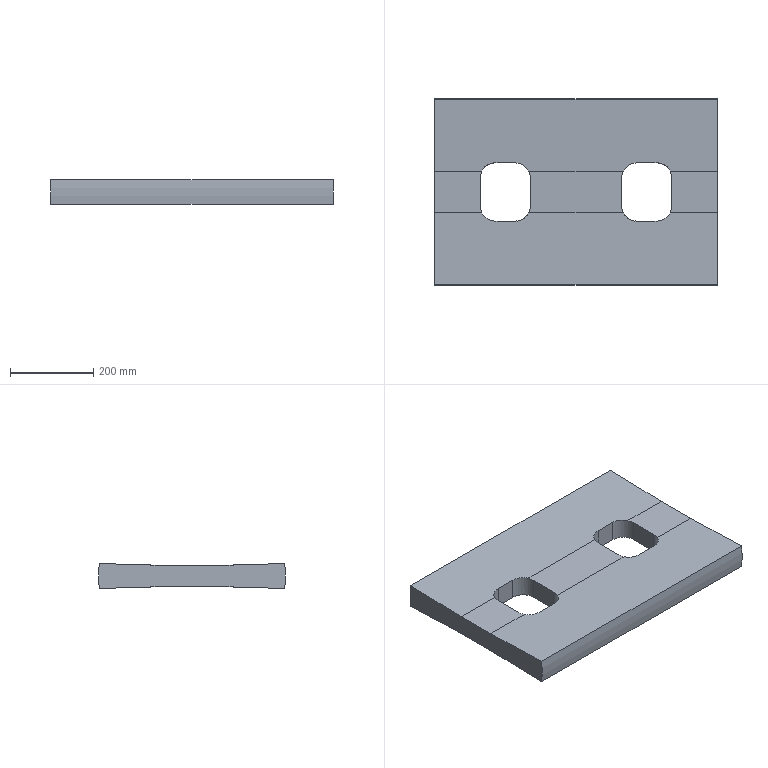Part | SolidWorks | features Extrusion 1, ICE 1, MirrorPattern 1 | 1 solid | 30 faces | box 680 x 450 x 60 mm | volume 14870230 mm3 | plane 20 | cylinder 10 | commonest cylinder face diameters 70 x8 450 x2
STEP:
#1=CARTESIAN_POINT('',(110.,-35.,25.));
#2=VERTEX_POINT('',#1);
#3=CARTESIAN_POINT('',(113.377,-50.,25.));
#4=VERTEX_POINT('',#3);
#5=CARTESIAN_POINT('',(145.,-35.,25.));
#6=DIRECTION('',(0.,0.,1.));
#7=DIRECTION('',(0.,1.,0.));
#8=AXIS2_PLACEMENT_3D('',#5,#6,#7);
#9=CIRCLE('',#8,35.);
#10=EDGE_CURVE('',#2,#4,#9,.T.);
#11=ORIENTED_EDGE('',*,*,#10,.F.);
#12=CARTESIAN_POINT('',(110.,35.,25.));
#13=VERTEX_POINT('',#12);
#14=CARTESIAN_POINT('',(110.,-50.,25.));
#15=DIRECTION('',(0.,-1.,0.));
#16=VECTOR('',#15,1000.);
#17=LINE('',#14,#16);
#18=EDGE_CURVE('',#13,#2,#17,.T.);
#19=ORIENTED_EDGE('',*,*,#18,.F.);
#20=CARTESIAN_POINT('',(113.377,50.,25.));
#21=VERTEX_POINT('',#20);
#22=CARTESIAN_POINT('',(145.,35.,25.));
#23=DIRECTION('',(0.,0.,1.));
#24=DIRECTION('',(0.,1.,0.));
#25=AXIS2_PLACEMENT_3D('',#22,#23,#24);
#26=CIRCLE('',#25,35.);
#27=EDGE_CURVE('',#21,#13,#26,.T.);
#28=ORIENTED_EDGE('',*,*,#27,.F.);
#29=CARTESIAN_POINT('',(-113.377,50.,25.));
#30=VERTEX_POINT('',#29);
#31=CARTESIAN_POINT('',(340.,50.,25.));
#32=DIRECTION('',(-1.,0.,0.));
#33=VECTOR('',#32,1000.);
#34=LINE('',#31,#33);
#35=EDGE_CURVE('',#21,#30,#34,.T.);
#36=ORIENTED_EDGE('',*,*,#35,.T.);
#37=CARTESIAN_POINT('',(-110.,35.,25.));
#38=VERTEX_POINT('',#37);
#39=CARTESIAN_POINT('',(-145.,35.,25.));
#40=DIRECTION('',(0.,0.,-1.));
#41=DIRECTION('',(0.,1.,0.));
#42=AXIS2_PLACEMENT_3D('',#39,#40,#41);
#43=CIRCLE('',#42,35.);
#44=EDGE_CURVE('',#30,#38,#43,.T.);
#45=ORIENTED_EDGE('',*,*,#44,.T.);
#46=CARTESIAN_POINT('',(-110.,-35.,25.));
#47=VERTEX_POINT('',#46);
#48=CARTESIAN_POINT('',(-110.,-50.,25.));
#49=DIRECTION('',(0.,-1.,0.));
#50=VECTOR('',#49,1000.);
#51=LINE('',#48,#50);
#52=EDGE_CURVE('',#38,#47,#51,.T.);
#53=ORIENTED_EDGE('',*,*,#52,.T.);
#54=CARTESIAN_POINT('',(-113.377,-50.,25.));
#55=VERTEX_POINT('',#54);
#56=CARTESIAN_POINT('',(-145.,-35.,25.));
#57=DIRECTION('',(0.,0.,-1.));
#58=DIRECTION('',(0.,1.,0.));
#59=AXIS2_PLACEMENT_3D('',#56,#57,#58);
#60=CIRCLE('',#59,35.);
#61=EDGE_CURVE('',#47,#55,#60,.T.);
#62=ORIENTED_EDGE('',*,*,#61,.T.);
#63=CARTESIAN_POINT('',(340.,-50.,25.));
#64=DIRECTION('',(-1.,0.,0.));
#65=VECTOR('',#64,1000.);
#66=LINE('',#63,#65);
#67=EDGE_CURVE('',#4,#55,#66,.T.);
#68=ORIENTED_EDGE('',*,*,#67,.F.);
#69=EDGE_LOOP('',(#11,#19,#28,#36,#45,#53,#62,#68));
#70=FACE_OUTER_BOUND('',#69,.T.);
#71=CARTESIAN_POINT('',(340.,-50.,25.));
#72=DIRECTION('',(0.,0.,-1.));
#73=DIRECTION('',(0.,1.,0.));
#74=AXIS2_PLACEMENT_3D('',#71,#72,#73);
#75=PLANE('',#74);
#76=ADVANCED_FACE('',(#70),#75,.F.);
#77=CARTESIAN_POINT('',(145.,-70.,25.578));
#78=VERTEX_POINT('',#77);
#79=CARTESIAN_POINT('',(113.377,-50.,25.));
#80=CARTESIAN_POINT('',(119.338,-62.566,25.363));
#81=CARTESIAN_POINT('',(131.092,-70.,25.578));
#82=CARTESIAN_POINT('',(145.,-70.,25.578));
#83=(BOUNDED_CURVE()B_SPLINE_CURVE(3,(#79,#80,#81,#82),.UNSPECIFIED.,.F.,.F.)B_SPLINE_CURVE_WITH_KNOTS((4,4),(5.155,6.283),.UNSPECIFIED.)CURVE()GEOMETRIC_REPRESENTATION_ITEM()RATIONAL_B_SPLINE_CURVE((1.,0.8968,0.8968,1.))REPRESENTATION_ITEM(''));
#84=EDGE_CURVE('',#4,#78,#83,.T.);
#85=ORIENTED_EDGE('',*,*,#84,.F.);
#86=ORIENTED_EDGE('',*,*,#67,.T.);
#87=CARTESIAN_POINT('',(-145.,-70.,25.578));
#88=VERTEX_POINT('',#87);
#89=CARTESIAN_POINT('',(-113.377,-50.,25.));
#90=CARTESIAN_POINT('',(-119.338,-62.566,25.363));
#91=CARTESIAN_POINT('',(-131.092,-70.,25.578));
#92=CARTESIAN_POINT('',(-145.,-70.,25.578));
#93=(BOUNDED_CURVE()B_SPLINE_CURVE(3,(#89,#90,#91,#92),.UNSPECIFIED.,.F.,.F.)B_SPLINE_CURVE_WITH_KNOTS((4,4),(5.155,6.283),.UNSPECIFIED.)CURVE()GEOMETRIC_REPRESENTATION_ITEM()RATIONAL_B_SPLINE_CURVE((1.,0.8968,0.8968,1.))REPRESENTATION_ITEM(''));
#94=EDGE_CURVE('',#55,#88,#93,.T.);
#95=ORIENTED_EDGE('',*,*,#94,.T.);
#96=CARTESIAN_POINT('',(-195.,-70.,25.578));
#97=VERTEX_POINT('',#96);
#98=CARTESIAN_POINT('',(340.,-70.,25.578));
#99=DIRECTION('',(-1.,0.,0.));
#100=VECTOR('',#99,1000.);
#101=LINE('',#98,#100);
#102=EDGE_CURVE('',#88,#97,#101,.T.);
#103=ORIENTED_EDGE('',*,*,#102,.T.);
#104=CARTESIAN_POINT('',(-226.623,-50.,25.));
#105=VERTEX_POINT('',#104);
#106=CARTESIAN_POINT('',(-195.,-70.,25.578));
#107=CARTESIAN_POINT('',(-208.908,-70.,25.578));
#108=CARTESIAN_POINT('',(-220.662,-62.566,25.363));
#109=CARTESIAN_POINT('',(-226.623,-50.,25.));
#110=(BOUNDED_CURVE()B_SPLINE_CURVE(3,(#106,#107,#108,#109),.UNSPECIFIED.,.F.,.F.)B_SPLINE_CURVE_WITH_KNOTS((4,4),(0.,1.128),.UNSPECIFIED.)CURVE()GEOMETRIC_REPRESENTATION_ITEM()RATIONAL_B_SPLINE_CURVE((1.,0.8968,0.8968,1.))REPRESENTATION_ITEM(''));
#111=EDGE_CURVE('',#97,#105,#110,.T.);
#112=ORIENTED_EDGE('',*,*,#111,.T.);
#113=CARTESIAN_POINT('',(-340.,-50.,25.));
#114=VERTEX_POINT('',#113);
#115=CARTESIAN_POINT('',(340.,-50.,25.));
#116=DIRECTION('',(-1.,0.,0.));
#117=VECTOR('',#116,1000.);
#118=LINE('',#115,#117);
#119=EDGE_CURVE('',#105,#114,#118,.T.);
#120=ORIENTED_EDGE('',*,*,#119,.T.);
#121=CARTESIAN_POINT('',(-340.,-222.991,30.));
#122=VERTEX_POINT('',#121);
#123=CARTESIAN_POINT('',(-340.,-50.,25.));
#124=DIRECTION('',(0.,-0.9996,0.02889));
#125=VECTOR('',#124,1000.);
#126=LINE('',#123,#125);
#127=EDGE_CURVE('',#114,#122,#126,.T.);
#128=ORIENTED_EDGE('',*,*,#127,.T.);
#129=CARTESIAN_POINT('',(340.,-222.991,30.));
#130=VERTEX_POINT('',#129);
#131=CARTESIAN_POINT('',(340.,-222.991,30.));
#132=DIRECTION('',(-1.,0.,0.));
#133=VECTOR('',#132,1000.);
#134=LINE('',#131,#133);
#135=EDGE_CURVE('',#130,#122,#134,.T.);
#136=ORIENTED_EDGE('',*,*,#135,.F.);
#137=CARTESIAN_POINT('',(340.,-50.,25.));
#138=VERTEX_POINT('',#137);
#139=CARTESIAN_POINT('',(340.,-50.,25.));
#140=DIRECTION('',(0.,-0.9996,0.02889));
#141=VECTOR('',#140,1000.);
#142=LINE('',#139,#141);
#143=EDGE_CURVE('',#138,#130,#142,.T.);
#144=ORIENTED_EDGE('',*,*,#143,.F.);
#145=CARTESIAN_POINT('',(226.623,-50.,25.));
#146=VERTEX_POINT('',#145);
#147=CARTESIAN_POINT('',(340.,-50.,25.));
#148=DIRECTION('',(-1.,0.,0.));
#149=VECTOR('',#148,1000.);
#150=LINE('',#147,#149);
#151=EDGE_CURVE('',#138,#146,#150,.T.);
#152=ORIENTED_EDGE('',*,*,#151,.T.);
#153=CARTESIAN_POINT('',(195.,-70.,25.578));
#154=VERTEX_POINT('',#153);
#155=CARTESIAN_POINT('',(195.,-70.,25.578));
#156=CARTESIAN_POINT('',(208.908,-70.,25.578));
#157=CARTESIAN_POINT('',(220.662,-62.566,25.363));
#158=CARTESIAN_POINT('',(226.623,-50.,25.));
#159=(BOUNDED_CURVE()B_SPLINE_CURVE(3,(#155,#156,#157,#158),.UNSPECIFIED.,.F.,.F.)B_SPLINE_CURVE_WITH_KNOTS((4,4),(0.,1.128),.UNSPECIFIED.)CURVE()GEOMETRIC_REPRESENTATION_ITEM()RATIONAL_B_SPLINE_CURVE((1.,0.8968,0.8968,1.))REPRESENTATION_ITEM(''));
#160=EDGE_CURVE('',#154,#146,#159,.T.);
#161=ORIENTED_EDGE('',*,*,#160,.F.);
#162=CARTESIAN_POINT('',(340.,-70.,25.578));
#163=DIRECTION('',(1.,0.,0.));
#164=VECTOR('',#163,1000.);
#165=LINE('',#162,#164);
#166=EDGE_CURVE('',#78,#154,#165,.T.);
#167=ORIENTED_EDGE('',*,*,#166,.F.);
#168=EDGE_LOOP('',(#85,#86,#95,#103,#112,#120,#128,#136,#144,#152,#161,#167));
#169=FACE_OUTER_BOUND('',#168,.T.);
#170=CARTESIAN_POINT('',(340.,-50.,25.));
#171=DIRECTION('',(0.,-0.02889,-0.9996));
#172=DIRECTION('',(0.,0.9996,-0.02889));
#173=AXIS2_PLACEMENT_3D('',#170,#171,#172);
#174=PLANE('',#173);
#175=ADVANCED_FACE('',(#169),#174,.F.);
#176=CARTESIAN_POINT('',(145.,-70.,-25.578));
#177=VERTEX_POINT('',#176);
#178=CARTESIAN_POINT('',(113.377,-50.,-25.));
#179=VERTEX_POINT('',#178);
#180=CARTESIAN_POINT('',(145.,-70.,-25.578));
#181=CARTESIAN_POINT('',(131.092,-70.,-25.578));
#182=CARTESIAN_POINT('',(119.338,-62.566,-25.363));
#183=CARTESIAN_POINT('',(113.377,-50.,-25.));
#184=(BOUNDED_CURVE()B_SPLINE_CURVE(3,(#180,#181,#182,#183),.UNSPECIFIED.,.F.,.T.)B_SPLINE_CURVE_WITH_KNOTS((4,4),(3.142,4.269),.UNSPECIFIED.)CURVE()GEOMETRIC_REPRESENTATION_ITEM()RATIONAL_B_SPLINE_CURVE((1.,0.8968,0.8968,1.))REPRESENTATION_ITEM(''));
#185=EDGE_CURVE('',#177,#179,#184,.T.);
#186=ORIENTED_EDGE('',*,*,#185,.F.);
#187=CARTESIAN_POINT('',(195.,-70.,-25.578));
#188=VERTEX_POINT('',#187);
#189=CARTESIAN_POINT('',(340.,-70.,-25.578));
#190=DIRECTION('',(-1.,0.,0.));
#191=VECTOR('',#190,1000.);
#192=LINE('',#189,#191);
#193=EDGE_CURVE('',#188,#177,#192,.T.);
#194=ORIENTED_EDGE('',*,*,#193,.F.);
#195=CARTESIAN_POINT('',(226.623,-50.,-25.));
#196=VERTEX_POINT('',#195);
#197=CARTESIAN_POINT('',(226.623,-50.,-25.));
#198=CARTESIAN_POINT('',(220.662,-62.566,-25.363));
#199=CARTESIAN_POINT('',(208.908,-70.,-25.578));
#200=CARTESIAN_POINT('',(195.,-70.,-25.578));
#201=(BOUNDED_CURVE()B_SPLINE_CURVE(3,(#197,#198,#199,#200),.UNSPECIFIED.,.F.,.F.)B_SPLINE_CURVE_WITH_KNOTS((4,4),(2.014,3.142),.UNSPECIFIED.)CURVE()GEOMETRIC_REPRESENTATION_ITEM()RATIONAL_B_SPLINE_CURVE((1.,0.8968,0.8968,1.))REPRESENTATION_ITEM(''));
#202=EDGE_CURVE('',#196,#188,#201,.T.);
#203=ORIENTED_EDGE('',*,*,#202,.F.);
#204=CARTESIAN_POINT('',(340.,-50.,-25.));
#205=VERTEX_POINT('',#204);
#206=CARTESIAN_POINT('',(340.,-50.,-25.));
#207=DIRECTION('',(-1.,0.,0.));
#208=VECTOR('',#207,1000.);
#209=LINE('',#206,#208);
#210=EDGE_CURVE('',#205,#196,#209,.T.);
#211=ORIENTED_EDGE('',*,*,#210,.F.);
#212=CARTESIAN_POINT('',(340.,-222.991,-30.));
#213=VERTEX_POINT('',#212);
#214=CARTESIAN_POINT('',(340.,-50.,-25.));
#215=DIRECTION('',(0.,0.9996,0.02889));
#216=VECTOR('',#215,1000.);
#217=LINE('',#214,#216);
#218=EDGE_CURVE('',#213,#205,#217,.T.);
#219=ORIENTED_EDGE('',*,*,#218,.F.);
#220=CARTESIAN_POINT('',(-340.,-222.991,-30.));
#221=VERTEX_POINT('',#220);
#222=CARTESIAN_POINT('',(340.,-222.991,-30.));
#223=DIRECTION('',(-1.,0.,0.));
#224=VECTOR('',#223,1000.);
#225=LINE('',#222,#224);
#226=EDGE_CURVE('',#213,#221,#225,.T.);
#227=ORIENTED_EDGE('',*,*,#226,.T.);
#228=CARTESIAN_POINT('',(-340.,-50.,-25.));
#229=VERTEX_POINT('',#228);
#230=CARTESIAN_POINT('',(-340.,-50.,-25.));
#231=DIRECTION('',(0.,0.9996,0.02889));
#232=VECTOR('',#231,1000.);
#233=LINE('',#230,#232);
#234=EDGE_CURVE('',#221,#229,#233,.T.);
#235=ORIENTED_EDGE('',*,*,#234,.T.);
#236=CARTESIAN_POINT('',(-226.623,-50.,-25.));
#237=VERTEX_POINT('',#236);
#238=CARTESIAN_POINT('',(340.,-50.,-25.));
#239=DIRECTION('',(-1.,0.,0.));
#240=VECTOR('',#239,1000.);
#241=LINE('',#238,#240);
#242=EDGE_CURVE('',#237,#229,#241,.T.);
#243=ORIENTED_EDGE('',*,*,#242,.F.);
#244=CARTESIAN_POINT('',(-195.,-70.,-25.578));
#245=VERTEX_POINT('',#244);
#246=CARTESIAN_POINT('',(-226.623,-50.,-25.));
#247=CARTESIAN_POINT('',(-220.662,-62.566,-25.363));
#248=CARTESIAN_POINT('',(-208.908,-70.,-25.578));
#249=CARTESIAN_POINT('',(-195.,-70.,-25.578));
#250=(BOUNDED_CURVE()B_SPLINE_CURVE(3,(#246,#247,#248,#249),.UNSPECIFIED.,.F.,.F.)B_SPLINE_CURVE_WITH_KNOTS((4,4),(2.014,3.142),.UNSPECIFIED.)CURVE()GEOMETRIC_REPRESENTATION_ITEM()RATIONAL_B_SPLINE_CURVE((1.,0.8968,0.8968,1.))REPRESENTATION_ITEM(''));
#251=EDGE_CURVE('',#237,#245,#250,.T.);
#252=ORIENTED_EDGE('',*,*,#251,.T.);
#253=CARTESIAN_POINT('',(-145.,-70.,-25.578));
#254=VERTEX_POINT('',#253);
#255=CARTESIAN_POINT('',(340.,-70.,-25.578));
#256=DIRECTION('',(1.,0.,0.));
#257=VECTOR('',#256,1000.);
#258=LINE('',#255,#257);
#259=EDGE_CURVE('',#245,#254,#258,.T.);
#260=ORIENTED_EDGE('',*,*,#259,.T.);
#261=CARTESIAN_POINT('',(-113.377,-50.,-25.));
#262=VERTEX_POINT('',#261);
#263=CARTESIAN_POINT('',(-145.,-70.,-25.578));
#264=CARTESIAN_POINT('',(-131.092,-70.,-25.578));
#265=CARTESIAN_POINT('',(-119.338,-62.566,-25.363));
#266=CARTESIAN_POINT('',(-113.377,-50.,-25.));
#267=(BOUNDED_CURVE()B_SPLINE_CURVE(3,(#263,#264,#265,#266),.UNSPECIFIED.,.F.,.T.)B_SPLINE_CURVE_WITH_KNOTS((4,4),(3.142,4.269),.UNSPECIFIED.)CURVE()GEOMETRIC_REPRESENTATION_ITEM()RATIONAL_B_SPLINE_CURVE((1.,0.8968,0.8968,1.))REPRESENTATION_ITEM(''));
#268=EDGE_CURVE('',#254,#262,#267,.T.);
#269=ORIENTED_EDGE('',*,*,#268,.T.);
#270=CARTESIAN_POINT('',(340.,-50.,-25.));
#271=DIRECTION('',(-1.,0.,0.));
#272=VECTOR('',#271,1000.);
#273=LINE('',#270,#272);
#274=EDGE_CURVE('',#179,#262,#273,.T.);
#275=ORIENTED_EDGE('',*,*,#274,.F.);
#276=EDGE_LOOP('',(#186,#194,#203,#211,#219,#227,#235,#243,#252,#260,#269,#275));
#277=FACE_OUTER_BOUND('',#276,.T.);
#278=CARTESIAN_POINT('',(340.,-50.,-25.));
#279=DIRECTION('',(0.,-0.02889,0.9996));
#280=DIRECTION('',(0.,-0.9996,-0.02889));
#281=AXIS2_PLACEMENT_3D('',#278,#279,#280);
#282=PLANE('',#281);
#283=ADVANCED_FACE('',(#277),#282,.F.);
#284=CARTESIAN_POINT('',(110.,-35.,-25.));
#285=VERTEX_POINT('',#284);
#286=CARTESIAN_POINT('',(145.,-35.,-25.));
#287=DIRECTION('',(0.,0.,-1.));
#288=DIRECTION('',(0.,-1.,0.));
#289=AXIS2_PLACEMENT_3D('',#286,#287,#288);
#290=CIRCLE('',#289,35.);
#291=EDGE_CURVE('',#179,#285,#290,.T.);
#292=ORIENTED_EDGE('',*,*,#291,.F.);
#293=ORIENTED_EDGE('',*,*,#274,.T.);
#294=CARTESIAN_POINT('',(-110.,-35.,-25.));
#295=VERTEX_POINT('',#294);
#296=CARTESIAN_POINT('',(-145.,-35.,-25.));
#297=DIRECTION('',(0.,0.,1.));
#298=DIRECTION('',(0.,-1.,0.));
#299=AXIS2_PLACEMENT_3D('',#296,#297,#298);
#300=CIRCLE('',#299,35.);
#301=EDGE_CURVE('',#262,#295,#300,.T.);
#302=ORIENTED_EDGE('',*,*,#301,.T.);
#303=CARTESIAN_POINT('',(-110.,35.,-25.));
#304=VERTEX_POINT('',#303);
#305=CARTESIAN_POINT('',(-110.,-50.,-25.));
#306=DIRECTION('',(0.,1.,0.));
#307=VECTOR('',#306,1000.);
#308=LINE('',#305,#307);
#309=EDGE_CURVE('',#295,#304,#308,.T.);
#310=ORIENTED_EDGE('',*,*,#309,.T.);
#311=CARTESIAN_POINT('',(-113.377,50.,-25.));
#312=VERTEX_POINT('',#311);
#313=CARTESIAN_POINT('',(-145.,35.,-25.));
#314=DIRECTION('',(0.,0.,1.));
#315=DIRECTION('',(0.,-1.,0.));
#316=AXIS2_PLACEMENT_3D('',#313,#314,#315);
#317=CIRCLE('',#316,35.);
#318=EDGE_CURVE('',#304,#312,#317,.T.);
#319=ORIENTED_EDGE('',*,*,#318,.T.);
#320=CARTESIAN_POINT('',(113.377,50.,-25.));
#321=VERTEX_POINT('',#320);
#322=CARTESIAN_POINT('',(340.,50.,-25.));
#323=DIRECTION('',(-1.,0.,0.));
#324=VECTOR('',#323,1000.);
#325=LINE('',#322,#324);
#326=EDGE_CURVE('',#321,#312,#325,.T.);
#327=ORIENTED_EDGE('',*,*,#326,.F.);
#328=CARTESIAN_POINT('',(110.,35.,-25.));
#329=VERTEX_POINT('',#328);
#330=CARTESIAN_POINT('',(145.,35.,-25.));
#331=DIRECTION('',(0.,0.,-1.));
#332=DIRECTION('',(0.,-1.,0.));
#333=AXIS2_PLACEMENT_3D('',#330,#331,#332);
#334=CIRCLE('',#333,35.);
#335=EDGE_CURVE('',#329,#321,#334,.T.);
#336=ORIENTED_EDGE('',*,*,#335,.F.);
#337=CARTESIAN_POINT('',(110.,-50.,-25.));
#338=DIRECTION('',(0.,1.,0.));
#339=VECTOR('',#338,1000.);
#340=LINE('',#337,#339);
#341=EDGE_CURVE('',#285,#329,#340,.T.);
#342=ORIENTED_EDGE('',*,*,#341,.F.);
#343=EDGE_LOOP('',(#292,#293,#302,#310,#319,#327,#336,#342));
#344=FACE_OUTER_BOUND('',#343,.T.);
#345=CARTESIAN_POINT('',(340.,-50.,-25.));
#346=DIRECTION('',(0.,0.,1.));
#347=DIRECTION('',(0.,-1.,0.));
#348=AXIS2_PLACEMENT_3D('',#345,#346,#347);
#349=PLANE('',#348);
#350=ADVANCED_FACE('',(#344),#349,.F.);
#351=ORIENTED_EDGE('',*,*,#119,.F.);
#352=CARTESIAN_POINT('',(-230.,-35.,25.));
#353=VERTEX_POINT('',#352);
#354=CARTESIAN_POINT('',(-195.,-35.,25.));
#355=DIRECTION('',(0.,0.,-1.));
#356=DIRECTION('',(0.,1.,0.));
#357=AXIS2_PLACEMENT_3D('',#354,#355,#356);
#358=CIRCLE('',#357,35.);
#359=EDGE_CURVE('',#105,#353,#358,.T.);
#360=ORIENTED_EDGE('',*,*,#359,.T.);
#361=CARTESIAN_POINT('',(-230.,35.,25.));
#362=VERTEX_POINT('',#361);
#363=CARTESIAN_POINT('',(-230.,-50.,25.));
#364=DIRECTION('',(0.,1.,0.));
#365=VECTOR('',#364,1000.);
#366=LINE('',#363,#365);
#367=EDGE_CURVE('',#353,#362,#366,.T.);
#368=ORIENTED_EDGE('',*,*,#367,.T.);
#369=CARTESIAN_POINT('',(-226.623,50.,25.));
#370=VERTEX_POINT('',#369);
#371=CARTESIAN_POINT('',(-195.,35.,25.));
#372=DIRECTION('',(0.,0.,-1.));
#373=DIRECTION('',(0.,1.,0.));
#374=AXIS2_PLACEMENT_3D('',#371,#372,#373);
#375=CIRCLE('',#374,35.);
#376=EDGE_CURVE('',#362,#370,#375,.T.);
#377=ORIENTED_EDGE('',*,*,#376,.T.);
#378=CARTESIAN_POINT('',(-340.,50.,25.));
#379=VERTEX_POINT('',#378);
#380=CARTESIAN_POINT('',(340.,50.,25.));
#381=DIRECTION('',(-1.,0.,0.));
#382=VECTOR('',#381,1000.);
#383=LINE('',#380,#382);
#384=EDGE_CURVE('',#370,#379,#383,.T.);
#385=ORIENTED_EDGE('',*,*,#384,.T.);
#386=CARTESIAN_POINT('',(-340.,-50.,25.));
#387=DIRECTION('',(0.,-1.,0.));
#388=VECTOR('',#387,1000.);
#389=LINE('',#386,#388);
#390=EDGE_CURVE('',#379,#114,#389,.T.);
#391=ORIENTED_EDGE('',*,*,#390,.T.);
#392=EDGE_LOOP('',(#351,#360,#368,#377,#385,#391));
#393=FACE_OUTER_BOUND('',#392,.T.);
#394=CARTESIAN_POINT('',(340.,-50.,25.));
#395=DIRECTION('',(0.,0.,-1.));
#396=DIRECTION('',(0.,1.,0.));
#397=AXIS2_PLACEMENT_3D('',#394,#395,#396);
#398=PLANE('',#397);
#399=ADVANCED_FACE('',(#393),#398,.F.);
#400=CARTESIAN_POINT('',(-230.,35.,-25.));
#401=VERTEX_POINT('',#400);
#402=CARTESIAN_POINT('',(-230.,-35.,-25.));
#403=VERTEX_POINT('',#402);
#404=CARTESIAN_POINT('',(-230.,-50.,-25.));
#405=DIRECTION('',(0.,-1.,0.));
#406=VECTOR('',#405,1000.);
#407=LINE('',#404,#406);
#408=EDGE_CURVE('',#401,#403,#407,.T.);
#409=ORIENTED_EDGE('',*,*,#408,.T.);
#410=CARTESIAN_POINT('',(-195.,-35.,-25.));
#411=DIRECTION('',(0.,0.,1.));
#412=DIRECTION('',(0.,-1.,0.));
#413=AXIS2_PLACEMENT_3D('',#410,#411,#412);
#414=CIRCLE('',#413,35.);
#415=EDGE_CURVE('',#403,#237,#414,.T.);
#416=ORIENTED_EDGE('',*,*,#415,.T.);
#417=ORIENTED_EDGE('',*,*,#242,.T.);
#418=CARTESIAN_POINT('',(-340.,50.,-25.));
#419=VERTEX_POINT('',#418);
#420=CARTESIAN_POINT('',(-340.,-50.,-25.));
#421=DIRECTION('',(0.,1.,0.));
#422=VECTOR('',#421,1000.);
#423=LINE('',#420,#422);
#424=EDGE_CURVE('',#229,#419,#423,.T.);
#425=ORIENTED_EDGE('',*,*,#424,.T.);
#426=CARTESIAN_POINT('',(-226.623,50.,-25.));
#427=VERTEX_POINT('',#426);
#428=CARTESIAN_POINT('',(340.,50.,-25.));
#429=DIRECTION('',(-1.,0.,0.));
#430=VECTOR('',#429,1000.);
#431=LINE('',#428,#430);
#432=EDGE_CURVE('',#427,#419,#431,.T.);
#433=ORIENTED_EDGE('',*,*,#432,.F.);
#434=CARTESIAN_POINT('',(-195.,35.,-25.));
#435=DIRECTION('',(0.,0.,1.));
#436=DIRECTION('',(0.,-1.,0.));
#437=AXIS2_PLACEMENT_3D('',#434,#435,#436);
#438=CIRCLE('',#437,35.);
#439=EDGE_CURVE('',#427,#401,#438,.T.);
#440=ORIENTED_EDGE('',*,*,#439,.T.);
#441=EDGE_LOOP('',(#409,#416,#417,#425,#433,#440));
#442=FACE_OUTER_BOUND('',#441,.T.);
#443=CARTESIAN_POINT('',(340.,-50.,-25.));
#444=DIRECTION('',(0.,0.,1.));
#445=DIRECTION('',(0.,-1.,0.));
#446=AXIS2_PLACEMENT_3D('',#443,#444,#445);
#447=PLANE('',#446);
#448=ADVANCED_FACE('',(#442),#447,.F.);
#449=CARTESIAN_POINT('',(145.,70.,-25.578));
#450=VERTEX_POINT('',#449);
#451=CARTESIAN_POINT('',(113.377,50.,-25.));
#452=CARTESIAN_POINT('',(119.338,62.566,-25.363));
#453=CARTESIAN_POINT('',(131.092,70.,-25.578));
#454=CARTESIAN_POINT('',(145.,70.,-25.578));
#455=(BOUNDED_CURVE()B_SPLINE_CURVE(3,(#451,#452,#453,#454),.UNSPECIFIED.,.F.,.T.)B_SPLINE_CURVE_WITH_KNOTS((4,4),(2.014,3.142),.UNSPECIFIED.)CURVE()GEOMETRIC_REPRESENTATION_ITEM()RATIONAL_B_SPLINE_CURVE((1.,0.8968,0.8968,1.))REPRESENTATION_ITEM(''));
#456=EDGE_CURVE('',#321,#450,#455,.T.);
#457=ORIENTED_EDGE('',*,*,#456,.F.);
#458=ORIENTED_EDGE('',*,*,#326,.T.);
#459=CARTESIAN_POINT('',(-145.,70.,-25.578));
#460=VERTEX_POINT('',#459);
#461=CARTESIAN_POINT('',(-113.377,50.,-25.));
#462=CARTESIAN_POINT('',(-119.338,62.566,-25.363));
#463=CARTESIAN_POINT('',(-131.092,70.,-25.578));
#464=CARTESIAN_POINT('',(-145.,70.,-25.578));
#465=(BOUNDED_CURVE()B_SPLINE_CURVE(3,(#461,#462,#463,#464),.UNSPECIFIED.,.F.,.F.)B_SPLINE_CURVE_WITH_KNOTS((4,4),(2.014,3.142),.UNSPECIFIED.)CURVE()GEOMETRIC_REPRESENTATION_ITEM()RATIONAL_B_SPLINE_CURVE((1.,0.8968,0.8968,1.))REPRESENTATION_ITEM(''));
#466=EDGE_CURVE('',#312,#460,#465,.T.);
#467=ORIENTED_EDGE('',*,*,#466,.T.);
#468=CARTESIAN_POINT('',(-195.,70.,-25.578));
#469=VERTEX_POINT('',#468);
#470=CARTESIAN_POINT('',(340.,70.,-25.578));
#471=DIRECTION('',(-1.,0.,0.));
#472=VECTOR('',#471,1000.);
#473=LINE('',#470,#472);
#474=EDGE_CURVE('',#460,#469,#473,.T.);
#475=ORIENTED_EDGE('',*,*,#474,.T.);
#476=CARTESIAN_POINT('',(-195.,70.,-25.578));
#477=CARTESIAN_POINT('',(-208.908,70.,-25.578));
#478=CARTESIAN_POINT('',(-220.662,62.566,-25.363));
#479=CARTESIAN_POINT('',(-226.623,50.,-25.));
#480=(BOUNDED_CURVE()B_SPLINE_CURVE(3,(#476,#477,#478,#479),.UNSPECIFIED.,.F.,.F.)B_SPLINE_CURVE_WITH_KNOTS((4,4),(3.142,4.269),.UNSPECIFIED.)CURVE()GEOMETRIC_REPRESENTATION_ITEM()RATIONAL_B_SPLINE_CURVE((1.,0.8968,0.8968,1.))REPRESENTATION_ITEM(''));
#481=EDGE_CURVE('',#469,#427,#480,.T.);
#482=ORIENTED_EDGE('',*,*,#481,.T.);
#483=ORIENTED_EDGE('',*,*,#432,.T.);
#484=CARTESIAN_POINT('',(-340.,222.991,-30.));
#485=VERTEX_POINT('',#484);
#486=CARTESIAN_POINT('',(-340.,50.,-25.));
#487=DIRECTION('',(0.,0.9996,-0.02889));
#488=VECTOR('',#487,1000.);
#489=LINE('',#486,#488);
#490=EDGE_CURVE('',#419,#485,#489,.T.);
#491=ORIENTED_EDGE('',*,*,#490,.T.);
#492=CARTESIAN_POINT('',(340.,222.991,-30.));
#493=VERTEX_POINT('',#492);
#494=CARTESIAN_POINT('',(340.,222.991,-30.));
#495=DIRECTION('',(-1.,0.,0.));
#496=VECTOR('',#495,1000.);
#497=LINE('',#494,#496);
#498=EDGE_CURVE('',#493,#485,#497,.T.);
#499=ORIENTED_EDGE('',*,*,#498,.F.);
#500=CARTESIAN_POINT('',(340.,50.,-25.));
#501=VERTEX_POINT('',#500);
#502=CARTESIAN_POINT('',(340.,50.,-25.));
#503=DIRECTION('',(0.,0.9996,-0.02889));
#504=VECTOR('',#503,1000.);
#505=LINE('',#502,#504);
#506=EDGE_CURVE('',#501,#493,#505,.T.);
#507=ORIENTED_EDGE('',*,*,#506,.F.);
#508=CARTESIAN_POINT('',(226.623,50.,-25.));
#509=VERTEX_POINT('',#508);
#510=CARTESIAN_POINT('',(340.,50.,-25.));
#511=DIRECTION('',(-1.,0.,0.));
#512=VECTOR('',#511,1000.);
#513=LINE('',#510,#512);
#514=EDGE_CURVE('',#501,#509,#513,.T.);
#515=ORIENTED_EDGE('',*,*,#514,.T.);
#516=CARTESIAN_POINT('',(195.,70.,-25.578));
#517=VERTEX_POINT('',#516);
#518=CARTESIAN_POINT('',(195.,70.,-25.578));
#519=CARTESIAN_POINT('',(208.908,70.,-25.578));
#520=CARTESIAN_POINT('',(220.662,62.566,-25.363));
#521=CARTESIAN_POINT('',(226.623,50.,-25.));
#522=(BOUNDED_CURVE()B_SPLINE_CURVE(3,(#518,#519,#520,#521),.UNSPECIFIED.,.F.,.T.)B_SPLINE_CURVE_WITH_KNOTS((4,4),(3.142,4.269),.UNSPECIFIED.)CURVE()GEOMETRIC_REPRESENTATION_ITEM()RATIONAL_B_SPLINE_CURVE((1.,0.8968,0.8968,1.))REPRESENTATION_ITEM(''));
#523=EDGE_CURVE('',#517,#509,#522,.T.);
#524=ORIENTED_EDGE('',*,*,#523,.F.);
#525=CARTESIAN_POINT('',(340.,70.,-25.578));
#526=DIRECTION('',(1.,0.,0.));
#527=VECTOR('',#526,1000.);
#528=LINE('',#525,#527);
#529=EDGE_CURVE('',#450,#517,#528,.T.);
#530=ORIENTED_EDGE('',*,*,#529,.F.);
#531=EDGE_LOOP('',(#457,#458,#467,#475,#482,#483,#491,#499,#507,#515,#524,#530));
#532=FACE_OUTER_BOUND('',#531,.T.);
#533=CARTESIAN_POINT('',(340.,50.,-25.));
#534=DIRECTION('',(0.,0.02889,0.9996));
#535=DIRECTION('',(0.,-0.9996,0.02889));
#536=AXIS2_PLACEMENT_3D('',#533,#534,#535);
#537=PLANE('',#536);
#538=ADVANCED_FACE('',(#532),#537,.F.);
#539=CARTESIAN_POINT('',(-340.,222.991,30.));
#540=VERTEX_POINT('',#539);
#541=CARTESIAN_POINT('',(-340.,0.,0.));
#542=DIRECTION('',(1.,0.,0.));
#543=DIRECTION('',(0.,0.,-1.));
#544=AXIS2_PLACEMENT_3D('',#541,#542,#543);
#545=CIRCLE('',#544,225.);
#546=EDGE_CURVE('',#485,#540,#545,.T.);
#547=ORIENTED_EDGE('',*,*,#546,.T.);
#548=CARTESIAN_POINT('',(340.,222.991,30.));
#549=VERTEX_POINT('',#548);
#550=CARTESIAN_POINT('',(340.,222.991,30.));
#551=DIRECTION('',(-1.,0.,0.));
#552=VECTOR('',#551,1000.);
#553=LINE('',#550,#552);
#554=EDGE_CURVE('',#549,#540,#553,.T.);
#555=ORIENTED_EDGE('',*,*,#554,.F.);
#556=CARTESIAN_POINT('',(340.,0.,0.));
#557=DIRECTION('',(1.,0.,0.));
#558=DIRECTION('',(0.,0.,-1.));
#559=AXIS2_PLACEMENT_3D('',#556,#557,#558);
#560=CIRCLE('',#559,225.);
#561=EDGE_CURVE('',#493,#549,#560,.T.);
#562=ORIENTED_EDGE('',*,*,#561,.F.);
#563=ORIENTED_EDGE('',*,*,#498,.T.);
#564=EDGE_LOOP('',(#547,#555,#562,#563));
#565=FACE_OUTER_BOUND('',#564,.T.);
#566=CARTESIAN_POINT('',(340.,0.,0.));
#567=DIRECTION('',(-1.,0.,0.));
#568=DIRECTION('',(0.,0.,1.));
#569=AXIS2_PLACEMENT_3D('',#566,#567,#568);
#570=CYLINDRICAL_SURFACE('',#569,225.);
#571=ADVANCED_FACE('',(#565),#570,.T.);
#572=CARTESIAN_POINT('',(145.,70.,25.578));
#573=VERTEX_POINT('',#572);
#574=CARTESIAN_POINT('',(145.,70.,25.578));
#575=CARTESIAN_POINT('',(131.092,70.,25.578));
#576=CARTESIAN_POINT('',(119.338,62.566,25.363));
#577=CARTESIAN_POINT('',(113.377,50.,25.));
#578=(BOUNDED_CURVE()B_SPLINE_CURVE(3,(#574,#575,#576,#577),.UNSPECIFIED.,.F.,.F.)B_SPLINE_CURVE_WITH_KNOTS((4,4),(0.,1.128),.UNSPECIFIED.)CURVE()GEOMETRIC_REPRESENTATION_ITEM()RATIONAL_B_SPLINE_CURVE((1.,0.8968,0.8968,1.))REPRESENTATION_ITEM(''));
#579=EDGE_CURVE('',#573,#21,#578,.T.);
#580=ORIENTED_EDGE('',*,*,#579,.F.);
#581=CARTESIAN_POINT('',(195.,70.,25.578));
#582=VERTEX_POINT('',#581);
#583=CARTESIAN_POINT('',(340.,70.,25.578));
#584=DIRECTION('',(-1.,0.,0.));
#585=VECTOR('',#584,1000.);
#586=LINE('',#583,#585);
#587=EDGE_CURVE('',#582,#573,#586,.T.);
#588=ORIENTED_EDGE('',*,*,#587,.F.);
#589=CARTESIAN_POINT('',(226.623,50.,25.));
#590=VERTEX_POINT('',#589);
#591=CARTESIAN_POINT('',(226.623,50.,25.));
#592=CARTESIAN_POINT('',(220.662,62.566,25.363));
#593=CARTESIAN_POINT('',(208.908,70.,25.578));
#594=CARTESIAN_POINT('',(195.,70.,25.578));
#595=(BOUNDED_CURVE()B_SPLINE_CURVE(3,(#591,#592,#593,#594),.UNSPECIFIED.,.F.,.F.)B_SPLINE_CURVE_WITH_KNOTS((4,4),(5.155,6.283),.UNSPECIFIED.)CURVE()GEOMETRIC_REPRESENTATION_ITEM()RATIONAL_B_SPLINE_CURVE((1.,0.8968,0.8968,1.))REPRESENTATION_ITEM(''));
#596=EDGE_CURVE('',#590,#582,#595,.T.);
#597=ORIENTED_EDGE('',*,*,#596,.F.);
#598=CARTESIAN_POINT('',(340.,50.,25.));
#599=VERTEX_POINT('',#598);
#600=CARTESIAN_POINT('',(340.,50.,25.));
#601=DIRECTION('',(-1.,0.,0.));
#602=VECTOR('',#601,1000.);
#603=LINE('',#600,#602);
#604=EDGE_CURVE('',#599,#590,#603,.T.);
#605=ORIENTED_EDGE('',*,*,#604,.F.);
#606=CARTESIAN_POINT('',(340.,50.,25.));
#607=DIRECTION('',(0.,-0.9996,-0.02889));
#608=VECTOR('',#607,1000.);
#609=LINE('',#606,#608);
#610=EDGE_CURVE('',#549,#599,#609,.T.);
#611=ORIENTED_EDGE('',*,*,#610,.F.);
#612=ORIENTED_EDGE('',*,*,#554,.T.);
#613=CARTESIAN_POINT('',(-340.,50.,25.));
#614=DIRECTION('',(0.,-0.9996,-0.02889));
#615=VECTOR('',#614,1000.);
#616=LINE('',#613,#615);
#617=EDGE_CURVE('',#540,#379,#616,.T.);
#618=ORIENTED_EDGE('',*,*,#617,.T.);
#619=ORIENTED_EDGE('',*,*,#384,.F.);
#620=CARTESIAN_POINT('',(-195.,70.,25.578));
#621=VERTEX_POINT('',#620);
#622=CARTESIAN_POINT('',(-226.623,50.,25.));
#623=CARTESIAN_POINT('',(-220.662,62.566,25.363));
#624=CARTESIAN_POINT('',(-208.908,70.,25.578));
#625=CARTESIAN_POINT('',(-195.,70.,25.578));
#626=(BOUNDED_CURVE()B_SPLINE_CURVE(3,(#622,#623,#624,#625),.UNSPECIFIED.,.F.,.F.)B_SPLINE_CURVE_WITH_KNOTS((4,4),(5.155,6.283),.UNSPECIFIED.)CURVE()GEOMETRIC_REPRESENTATION_ITEM()RATIONAL_B_SPLINE_CURVE((1.,0.8968,0.8968,1.))REPRESENTATION_ITEM(''));
#627=EDGE_CURVE('',#370,#621,#626,.T.);
#628=ORIENTED_EDGE('',*,*,#627,.T.);
#629=CARTESIAN_POINT('',(-145.,70.,25.578));
#630=VERTEX_POINT('',#629);
#631=CARTESIAN_POINT('',(340.,70.,25.578));
#632=DIRECTION('',(1.,0.,0.));
#633=VECTOR('',#632,1000.);
#634=LINE('',#631,#633);
#635=EDGE_CURVE('',#621,#630,#634,.T.);
#636=ORIENTED_EDGE('',*,*,#635,.T.);
#637=CARTESIAN_POINT('',(-145.,70.,25.578));
#638=CARTESIAN_POINT('',(-131.092,70.,25.578));
#639=CARTESIAN_POINT('',(-119.338,62.566,25.363));
#640=CARTESIAN_POINT('',(-113.377,50.,25.));
#641=(BOUNDED_CURVE()B_SPLINE_CURVE(3,(#637,#638,#639,#640),.UNSPECIFIED.,.F.,.F.)B_SPLINE_CURVE_WITH_KNOTS((4,4),(0.,1.128),.UNSPECIFIED.)CURVE()GEOMETRIC_REPRESENTATION_ITEM()RATIONAL_B_SPLINE_CURVE((1.,0.8968,0.8968,1.))REPRESENTATION_ITEM(''));
#642=EDGE_CURVE('',#630,#30,#641,.T.);
#643=ORIENTED_EDGE('',*,*,#642,.T.);
#644=ORIENTED_EDGE('',*,*,#35,.F.);
#645=EDGE_LOOP('',(#580,#588,#597,#605,#611,#612,#618,#619,#628,#636,#643,#644));
#646=FACE_OUTER_BOUND('',#645,.T.);
#647=CARTESIAN_POINT('',(340.,50.,25.));
#648=DIRECTION('',(0.,0.02889,-0.9996));
#649=DIRECTION('',(0.,0.9996,0.02889));
#650=AXIS2_PLACEMENT_3D('',#647,#648,#649);
#651=PLANE('',#650);
#652=ADVANCED_FACE('',(#646),#651,.F.);
#653=CARTESIAN_POINT('',(230.,35.,25.));
#654=VERTEX_POINT('',#653);
#655=CARTESIAN_POINT('',(195.,35.,25.));
#656=DIRECTION('',(0.,0.,1.));
#657=DIRECTION('',(0.,1.,0.));
#658=AXIS2_PLACEMENT_3D('',#655,#656,#657);
#659=CIRCLE('',#658,35.);
#660=EDGE_CURVE('',#654,#590,#659,.T.);
#661=ORIENTED_EDGE('',*,*,#660,.F.);
#662=CARTESIAN_POINT('',(230.,-35.,25.));
#663=VERTEX_POINT('',#662);
#664=CARTESIAN_POINT('',(230.,-50.,25.));
#665=DIRECTION('',(0.,1.,0.));
#666=VECTOR('',#665,1000.);
#667=LINE('',#664,#666);
#668=EDGE_CURVE('',#663,#654,#667,.T.);
#669=ORIENTED_EDGE('',*,*,#668,.F.);
#670=CARTESIAN_POINT('',(195.,-35.,25.));
#671=DIRECTION('',(0.,0.,1.));
#672=DIRECTION('',(0.,1.,0.));
#673=AXIS2_PLACEMENT_3D('',#670,#671,#672);
#674=CIRCLE('',#673,35.);
#675=EDGE_CURVE('',#146,#663,#674,.T.);
#676=ORIENTED_EDGE('',*,*,#675,.F.);
#677=ORIENTED_EDGE('',*,*,#151,.F.);
#678=CARTESIAN_POINT('',(340.,-50.,25.));
#679=DIRECTION('',(0.,-1.,0.));
#680=VECTOR('',#679,1000.);
#681=LINE('',#678,#680);
#682=EDGE_CURVE('',#599,#138,#681,.T.);
#683=ORIENTED_EDGE('',*,*,#682,.F.);
#684=ORIENTED_EDGE('',*,*,#604,.T.);
#685=EDGE_LOOP('',(#661,#669,#676,#677,#683,#684));
#686=FACE_OUTER_BOUND('',#685,.T.);
#687=CARTESIAN_POINT('',(340.,-50.,25.));
#688=DIRECTION('',(0.,0.,-1.));
#689=DIRECTION('',(0.,1.,0.));
#690=AXIS2_PLACEMENT_3D('',#687,#688,#689);
#691=PLANE('',#690);
#692=ADVANCED_FACE('',(#686),#691,.F.);
#693=CARTESIAN_POINT('',(-340.,0.,0.));
#694=DIRECTION('',(1.,0.,0.));
#695=DIRECTION('',(0.,0.,-1.));
#696=AXIS2_PLACEMENT_3D('',#693,#694,#695);
#697=CIRCLE('',#696,225.);
#698=EDGE_CURVE('',#122,#221,#697,.T.);
#699=ORIENTED_EDGE('',*,*,#698,.T.);
#700=ORIENTED_EDGE('',*,*,#226,.F.);
#701=CARTESIAN_POINT('',(340.,0.,0.));
#702=DIRECTION('',(1.,0.,0.));
#703=DIRECTION('',(0.,0.,-1.));
#704=AXIS2_PLACEMENT_3D('',#701,#702,#703);
#705=CIRCLE('',#704,225.);
#706=EDGE_CURVE('',#130,#213,#705,.T.);
#707=ORIENTED_EDGE('',*,*,#706,.F.);
#708=ORIENTED_EDGE('',*,*,#135,.T.);
#709=EDGE_LOOP('',(#699,#700,#707,#708));
#710=FACE_OUTER_BOUND('',#709,.T.);
#711=CARTESIAN_POINT('',(340.,0.,0.));
#712=DIRECTION('',(-1.,0.,0.));
#713=DIRECTION('',(0.,0.,1.));
#714=AXIS2_PLACEMENT_3D('',#711,#712,#713);
#715=CYLINDRICAL_SURFACE('',#714,225.);
#716=ADVANCED_FACE('',(#710),#715,.T.);
#717=CARTESIAN_POINT('',(230.,35.,-25.));
#718=VERTEX_POINT('',#717);
#719=CARTESIAN_POINT('',(195.,35.,-25.));
#720=DIRECTION('',(0.,0.,-1.));
#721=DIRECTION('',(0.,-1.,0.));
#722=AXIS2_PLACEMENT_3D('',#719,#720,#721);
#723=CIRCLE('',#722,35.);
#724=EDGE_CURVE('',#509,#718,#723,.T.);
#725=ORIENTED_EDGE('',*,*,#724,.F.);
#726=ORIENTED_EDGE('',*,*,#514,.F.);
#727=CARTESIAN_POINT('',(340.,-50.,-25.));
#728=DIRECTION('',(0.,1.,0.));
#729=VECTOR('',#728,1000.);
#730=LINE('',#727,#729);
#731=EDGE_CURVE('',#205,#501,#730,.T.);
#732=ORIENTED_EDGE('',*,*,#731,.F.);
#733=ORIENTED_EDGE('',*,*,#210,.T.);
#734=CARTESIAN_POINT('',(230.,-35.,-25.));
#735=VERTEX_POINT('',#734);
#736=CARTESIAN_POINT('',(195.,-35.,-25.));
#737=DIRECTION('',(0.,0.,-1.));
#738=DIRECTION('',(0.,-1.,0.));
#739=AXIS2_PLACEMENT_3D('',#736,#737,#738);
#740=CIRCLE('',#739,35.);
#741=EDGE_CURVE('',#735,#196,#740,.T.);
#742=ORIENTED_EDGE('',*,*,#741,.F.);
#743=CARTESIAN_POINT('',(230.,-50.,-25.));
#744=DIRECTION('',(0.,-1.,0.));
#745=VECTOR('',#744,1000.);
#746=LINE('',#743,#745);
#747=EDGE_CURVE('',#718,#735,#746,.T.);
#748=ORIENTED_EDGE('',*,*,#747,.F.);
#749=EDGE_LOOP('',(#725,#726,#732,#733,#742,#748));
#750=FACE_OUTER_BOUND('',#749,.T.);
#751=CARTESIAN_POINT('',(340.,-50.,-25.));
#752=DIRECTION('',(0.,0.,1.));
#753=DIRECTION('',(0.,-1.,0.));
#754=AXIS2_PLACEMENT_3D('',#751,#752,#753);
#755=PLANE('',#754);
#756=ADVANCED_FACE('',(#750),#755,.F.);
#757=ORIENTED_EDGE('',*,*,#506,.T.);
#758=ORIENTED_EDGE('',*,*,#561,.T.);
#759=ORIENTED_EDGE('',*,*,#610,.T.);
#760=ORIENTED_EDGE('',*,*,#682,.T.);
#761=ORIENTED_EDGE('',*,*,#143,.T.);
#762=ORIENTED_EDGE('',*,*,#706,.T.);
#763=ORIENTED_EDGE('',*,*,#218,.T.);
#764=ORIENTED_EDGE('',*,*,#731,.T.);
#765=EDGE_LOOP('',(#757,#758,#759,#760,#761,#762,#763,#764));
#766=FACE_OUTER_BOUND('',#765,.T.);
#767=CARTESIAN_POINT('',(340.,0.,0.));
#768=DIRECTION('',(1.,0.,0.));
#769=DIRECTION('',(0.,0.,-1.));
#770=AXIS2_PLACEMENT_3D('',#767,#768,#769);
#771=PLANE('',#770);
#772=ADVANCED_FACE('',(#766),#771,.T.);
#773=ORIENTED_EDGE('',*,*,#490,.F.);
#774=ORIENTED_EDGE('',*,*,#424,.F.);
#775=ORIENTED_EDGE('',*,*,#234,.F.);
#776=ORIENTED_EDGE('',*,*,#698,.F.);
#777=ORIENTED_EDGE('',*,*,#127,.F.);
#778=ORIENTED_EDGE('',*,*,#390,.F.);
#779=ORIENTED_EDGE('',*,*,#617,.F.);
#780=ORIENTED_EDGE('',*,*,#546,.F.);
#781=EDGE_LOOP('',(#773,#774,#775,#776,#777,#778,#779,#780));
#782=FACE_OUTER_BOUND('',#781,.T.);
#783=CARTESIAN_POINT('',(-340.,0.,0.));
#784=DIRECTION('',(1.,0.,0.));
#785=DIRECTION('',(0.,0.,-1.));
#786=AXIS2_PLACEMENT_3D('',#783,#784,#785);
#787=PLANE('',#786);
#788=ADVANCED_FACE('',(#782),#787,.F.);
#789=CARTESIAN_POINT('',(-145.,70.,-30.));
#790=DIRECTION('',(0.,0.,1.));
#791=VECTOR('',#790,1000.);
#792=LINE('',#789,#791);
#793=EDGE_CURVE('',#460,#630,#792,.T.);
#794=ORIENTED_EDGE('',*,*,#793,.T.);
#795=ORIENTED_EDGE('',*,*,#635,.F.);
#796=CARTESIAN_POINT('',(-195.,70.,-30.));
#797=DIRECTION('',(0.,0.,1.));
#798=VECTOR('',#797,1000.);
#799=LINE('',#796,#798);
#800=EDGE_CURVE('',#469,#621,#799,.T.);
#801=ORIENTED_EDGE('',*,*,#800,.F.);
#802=ORIENTED_EDGE('',*,*,#474,.F.);
#803=EDGE_LOOP('',(#794,#795,#801,#802));
#804=FACE_OUTER_BOUND('',#803,.T.);
#805=CARTESIAN_POINT('',(-145.,70.,-30.));
#806=DIRECTION('',(0.,1.,0.));
#807=DIRECTION('',(-1.,0.,0.));
#808=AXIS2_PLACEMENT_3D('',#805,#806,#807);
#809=PLANE('',#808);
#810=ADVANCED_FACE('',(#804),#809,.F.);
#811=CARTESIAN_POINT('',(-145.,-70.,-30.));
#812=DIRECTION('',(0.,0.,1.));
#813=VECTOR('',#812,1000.);
#814=LINE('',#811,#813);
#815=EDGE_CURVE('',#254,#88,#814,.T.);
#816=ORIENTED_EDGE('',*,*,#815,.F.);
#817=ORIENTED_EDGE('',*,*,#259,.F.);
#818=CARTESIAN_POINT('',(-195.,-70.,-30.));
#819=DIRECTION('',(0.,0.,1.));
#820=VECTOR('',#819,1000.);
#821=LINE('',#818,#820);
#822=EDGE_CURVE('',#245,#97,#821,.T.);
#823=ORIENTED_EDGE('',*,*,#822,.T.);
#824=ORIENTED_EDGE('',*,*,#102,.F.);
#825=EDGE_LOOP('',(#816,#817,#823,#824));
#826=FACE_OUTER_BOUND('',#825,.T.);
#827=CARTESIAN_POINT('',(-145.,-70.,-30.));
#828=DIRECTION('',(0.,-1.,0.));
#829=DIRECTION('',(1.,0.,0.));
#830=AXIS2_PLACEMENT_3D('',#827,#828,#829);
#831=PLANE('',#830);
#832=ADVANCED_FACE('',(#826),#831,.F.);
#833=CARTESIAN_POINT('',(-110.,-35.,-30.));
#834=DIRECTION('',(0.,0.,1.));
#835=VECTOR('',#834,1000.);
#836=LINE('',#833,#835);
#837=EDGE_CURVE('',#295,#47,#836,.T.);
#838=ORIENTED_EDGE('',*,*,#837,.F.);
#839=ORIENTED_EDGE('',*,*,#301,.F.);
#840=ORIENTED_EDGE('',*,*,#268,.F.);
#841=ORIENTED_EDGE('',*,*,#815,.T.);
#842=ORIENTED_EDGE('',*,*,#94,.F.);
#843=ORIENTED_EDGE('',*,*,#61,.F.);
#844=EDGE_LOOP('',(#838,#839,#840,#841,#842,#843));
#845=FACE_OUTER_BOUND('',#844,.T.);
#846=CARTESIAN_POINT('',(-145.,-35.,-30.));
#847=DIRECTION('',(0.,0.,1.));
#848=DIRECTION('',(1.,0.,0.));
#849=AXIS2_PLACEMENT_3D('',#846,#847,#848);
#850=CYLINDRICAL_SURFACE('',#849,35.);
#851=ADVANCED_FACE('',(#845),#850,.F.);
#852=ORIENTED_EDGE('',*,*,#111,.F.);
#853=ORIENTED_EDGE('',*,*,#822,.F.);
#854=ORIENTED_EDGE('',*,*,#251,.F.);
#855=ORIENTED_EDGE('',*,*,#415,.F.);
#856=CARTESIAN_POINT('',(-230.,-35.,-30.));
#857=DIRECTION('',(0.,0.,1.));
#858=VECTOR('',#857,1000.);
#859=LINE('',#856,#858);
#860=EDGE_CURVE('',#403,#353,#859,.T.);
#861=ORIENTED_EDGE('',*,*,#860,.T.);
#862=ORIENTED_EDGE('',*,*,#359,.F.);
#863=EDGE_LOOP('',(#852,#853,#854,#855,#861,#862));
#864=FACE_OUTER_BOUND('',#863,.T.);
#865=CARTESIAN_POINT('',(-195.,-35.,-30.));
#866=DIRECTION('',(0.,0.,1.));
#867=DIRECTION('',(1.,0.,0.));
#868=AXIS2_PLACEMENT_3D('',#865,#866,#867);
#869=CYLINDRICAL_SURFACE('',#868,35.);
#870=ADVANCED_FACE('',(#864),#869,.F.);
#871=ORIENTED_EDGE('',*,*,#860,.F.);
#872=ORIENTED_EDGE('',*,*,#408,.F.);
#873=CARTESIAN_POINT('',(-230.,35.,-30.));
#874=DIRECTION('',(0.,0.,1.));
#875=VECTOR('',#874,1000.);
#876=LINE('',#873,#875);
#877=EDGE_CURVE('',#401,#362,#876,.T.);
#878=ORIENTED_EDGE('',*,*,#877,.T.);
#879=ORIENTED_EDGE('',*,*,#367,.F.);
#880=EDGE_LOOP('',(#871,#872,#878,#879));
#881=FACE_OUTER_BOUND('',#880,.T.);
#882=CARTESIAN_POINT('',(-230.,-35.,-30.));
#883=DIRECTION('',(-1.,0.,0.));
#884=DIRECTION('',(0.,-1.,0.));
#885=AXIS2_PLACEMENT_3D('',#882,#883,#884);
#886=PLANE('',#885);
#887=ADVANCED_FACE('',(#881),#886,.F.);
#888=ORIENTED_EDGE('',*,*,#376,.F.);
#889=ORIENTED_EDGE('',*,*,#877,.F.);
#890=ORIENTED_EDGE('',*,*,#439,.F.);
#891=ORIENTED_EDGE('',*,*,#481,.F.);
#892=ORIENTED_EDGE('',*,*,#800,.T.);
#893=ORIENTED_EDGE('',*,*,#627,.F.);
#894=EDGE_LOOP('',(#888,#889,#890,#891,#892,#893));
#895=FACE_OUTER_BOUND('',#894,.T.);
#896=CARTESIAN_POINT('',(-195.,35.,-30.));
#897=DIRECTION('',(0.,0.,1.));
#898=DIRECTION('',(1.,0.,0.));
#899=AXIS2_PLACEMENT_3D('',#896,#897,#898);
#900=CYLINDRICAL_SURFACE('',#899,35.);
#901=ADVANCED_FACE('',(#895),#900,.F.);
#902=ORIENTED_EDGE('',*,*,#793,.F.);
#903=ORIENTED_EDGE('',*,*,#466,.F.);
#904=ORIENTED_EDGE('',*,*,#318,.F.);
#905=CARTESIAN_POINT('',(-110.,35.,-30.));
#906=DIRECTION('',(0.,0.,1.));
#907=VECTOR('',#906,1000.);
#908=LINE('',#905,#907);
#909=EDGE_CURVE('',#304,#38,#908,.T.);
#910=ORIENTED_EDGE('',*,*,#909,.T.);
#911=ORIENTED_EDGE('',*,*,#44,.F.);
#912=ORIENTED_EDGE('',*,*,#642,.F.);
#913=EDGE_LOOP('',(#902,#903,#904,#910,#911,#912));
#914=FACE_OUTER_BOUND('',#913,.T.);
#915=CARTESIAN_POINT('',(-145.,35.,-30.));
#916=DIRECTION('',(0.,0.,1.));
#917=DIRECTION('',(1.,0.,0.));
#918=AXIS2_PLACEMENT_3D('',#915,#916,#917);
#919=CYLINDRICAL_SURFACE('',#918,35.);
#920=ADVANCED_FACE('',(#914),#919,.F.);
#921=ORIENTED_EDGE('',*,*,#909,.F.);
#922=ORIENTED_EDGE('',*,*,#309,.F.);
#923=ORIENTED_EDGE('',*,*,#837,.T.);
#924=ORIENTED_EDGE('',*,*,#52,.F.);
#925=EDGE_LOOP('',(#921,#922,#923,#924));
#926=FACE_OUTER_BOUND('',#925,.T.);
#927=CARTESIAN_POINT('',(-110.,-35.,-30.));
#928=DIRECTION('',(1.,0.,0.));
#929=DIRECTION('',(0.,1.,0.));
#930=AXIS2_PLACEMENT_3D('',#927,#928,#929);
#931=PLANE('',#930);
#932=ADVANCED_FACE('',(#926),#931,.F.);
#933=ORIENTED_EDGE('',*,*,#529,.T.);
#934=CARTESIAN_POINT('',(195.,70.,-30.));
#935=DIRECTION('',(0.,0.,1.));
#936=VECTOR('',#935,1000.);
#937=LINE('',#934,#936);
#938=EDGE_CURVE('',#517,#582,#937,.T.);
#939=ORIENTED_EDGE('',*,*,#938,.T.);
#940=ORIENTED_EDGE('',*,*,#587,.T.);
#941=CARTESIAN_POINT('',(145.,70.,-30.));
#942=DIRECTION('',(0.,0.,1.));
#943=VECTOR('',#942,1000.);
#944=LINE('',#941,#943);
#945=EDGE_CURVE('',#450,#573,#944,.T.);
#946=ORIENTED_EDGE('',*,*,#945,.F.);
#947=EDGE_LOOP('',(#933,#939,#940,#946));
#948=FACE_OUTER_BOUND('',#947,.T.);
#949=CARTESIAN_POINT('',(145.,70.,-30.));
#950=DIRECTION('',(0.,-1.,0.));
#951=DIRECTION('',(1.,0.,0.));
#952=AXIS2_PLACEMENT_3D('',#949,#950,#951);
#953=PLANE('',#952);
#954=ADVANCED_FACE('',(#948),#953,.T.);
#955=ORIENTED_EDGE('',*,*,#166,.T.);
#956=CARTESIAN_POINT('',(195.,-70.,-30.));
#957=DIRECTION('',(0.,0.,1.));
#958=VECTOR('',#957,1000.);
#959=LINE('',#956,#958);
#960=EDGE_CURVE('',#188,#154,#959,.T.);
#961=ORIENTED_EDGE('',*,*,#960,.F.);
#962=ORIENTED_EDGE('',*,*,#193,.T.);
#963=CARTESIAN_POINT('',(145.,-70.,-30.));
#964=DIRECTION('',(0.,0.,1.));
#965=VECTOR('',#964,1000.);
#966=LINE('',#963,#965);
#967=EDGE_CURVE('',#177,#78,#966,.T.);
#968=ORIENTED_EDGE('',*,*,#967,.T.);
#969=EDGE_LOOP('',(#955,#961,#962,#968));
#970=FACE_OUTER_BOUND('',#969,.T.);
#971=CARTESIAN_POINT('',(145.,-70.,-30.));
#972=DIRECTION('',(0.,1.,0.));
#973=DIRECTION('',(-1.,0.,0.));
#974=AXIS2_PLACEMENT_3D('',#971,#972,#973);
#975=PLANE('',#974);
#976=ADVANCED_FACE('',(#970),#975,.T.);
#977=ORIENTED_EDGE('',*,*,#10,.T.);
#978=ORIENTED_EDGE('',*,*,#84,.T.);
#979=ORIENTED_EDGE('',*,*,#967,.F.);
#980=ORIENTED_EDGE('',*,*,#185,.T.);
#981=ORIENTED_EDGE('',*,*,#291,.T.);
#982=CARTESIAN_POINT('',(110.,-35.,-30.));
#983=DIRECTION('',(0.,0.,1.));
#984=VECTOR('',#983,1000.);
#985=LINE('',#982,#984);
#986=EDGE_CURVE('',#285,#2,#985,.T.);
#987=ORIENTED_EDGE('',*,*,#986,.T.);
#988=EDGE_LOOP('',(#977,#978,#979,#980,#981,#987));
#989=FACE_OUTER_BOUND('',#988,.T.);
#990=CARTESIAN_POINT('',(145.,-35.,-30.));
#991=DIRECTION('',(0.,0.,1.));
#992=DIRECTION('',(1.,0.,0.));
#993=AXIS2_PLACEMENT_3D('',#990,#991,#992);
#994=CYLINDRICAL_SURFACE('',#993,35.);
#995=ADVANCED_FACE('',(#989),#994,.F.);
#996=ORIENTED_EDGE('',*,*,#18,.T.);
#997=ORIENTED_EDGE('',*,*,#986,.F.);
#998=ORIENTED_EDGE('',*,*,#341,.T.);
#999=CARTESIAN_POINT('',(110.,35.,-30.));
#1000=DIRECTION('',(0.,0.,1.));
#1001=VECTOR('',#1000,1000.);
#1002=LINE('',#999,#1001);
#1003=EDGE_CURVE('',#329,#13,#1002,.T.);
#1004=ORIENTED_EDGE('',*,*,#1003,.T.);
#1005=EDGE_LOOP('',(#996,#997,#998,#1004));
#1006=FACE_OUTER_BOUND('',#1005,.T.);
#1007=CARTESIAN_POINT('',(110.,-35.,-30.));
#1008=DIRECTION('',(1.,0.,0.));
#1009=DIRECTION('',(0.,1.,0.));
#1010=AXIS2_PLACEMENT_3D('',#1007,#1008,#1009);
#1011=PLANE('',#1010);
#1012=ADVANCED_FACE('',(#1006),#1011,.T.);
#1013=ORIENTED_EDGE('',*,*,#579,.T.);
#1014=ORIENTED_EDGE('',*,*,#27,.T.);
#1015=ORIENTED_EDGE('',*,*,#1003,.F.);
#1016=ORIENTED_EDGE('',*,*,#335,.T.);
#1017=ORIENTED_EDGE('',*,*,#456,.T.);
#1018=ORIENTED_EDGE('',*,*,#945,.T.);
#1019=EDGE_LOOP('',(#1013,#1014,#1015,#1016,#1017,#1018));
#1020=FACE_OUTER_BOUND('',#1019,.T.);
#1021=CARTESIAN_POINT('',(145.,35.,-30.));
#1022=DIRECTION('',(0.,0.,1.));
#1023=DIRECTION('',(1.,0.,0.));
#1024=AXIS2_PLACEMENT_3D('',#1021,#1022,#1023);
#1025=CYLINDRICAL_SURFACE('',#1024,35.);
#1026=ADVANCED_FACE('',(#1020),#1025,.F.);
#1027=ORIENTED_EDGE('',*,*,#596,.T.);
#1028=ORIENTED_EDGE('',*,*,#938,.F.);
#1029=ORIENTED_EDGE('',*,*,#523,.T.);
#1030=ORIENTED_EDGE('',*,*,#724,.T.);
#1031=CARTESIAN_POINT('',(230.,35.,-30.));
#1032=DIRECTION('',(0.,0.,1.));
#1033=VECTOR('',#1032,1000.);
#1034=LINE('',#1031,#1033);
#1035=EDGE_CURVE('',#718,#654,#1034,.T.);
#1036=ORIENTED_EDGE('',*,*,#1035,.T.);
#1037=ORIENTED_EDGE('',*,*,#660,.T.);
#1038=EDGE_LOOP('',(#1027,#1028,#1029,#1030,#1036,#1037));
#1039=FACE_OUTER_BOUND('',#1038,.T.);
#1040=CARTESIAN_POINT('',(195.,35.,-30.));
#1041=DIRECTION('',(0.,0.,1.));
#1042=DIRECTION('',(1.,0.,0.));
#1043=AXIS2_PLACEMENT_3D('',#1040,#1041,#1042);
#1044=CYLINDRICAL_SURFACE('',#1043,35.);
#1045=ADVANCED_FACE('',(#1039),#1044,.F.);
#1046=ORIENTED_EDGE('',*,*,#668,.T.);
#1047=ORIENTED_EDGE('',*,*,#1035,.F.);
#1048=ORIENTED_EDGE('',*,*,#747,.T.);
#1049=CARTESIAN_POINT('',(230.,-35.,-30.));
#1050=DIRECTION('',(0.,0.,1.));
#1051=VECTOR('',#1050,1000.);
#1052=LINE('',#1049,#1051);
#1053=EDGE_CURVE('',#735,#663,#1052,.T.);
#1054=ORIENTED_EDGE('',*,*,#1053,.T.);
#1055=EDGE_LOOP('',(#1046,#1047,#1048,#1054));
#1056=FACE_OUTER_BOUND('',#1055,.T.);
#1057=CARTESIAN_POINT('',(230.,-35.,-30.));
#1058=DIRECTION('',(-1.,0.,0.));
#1059=DIRECTION('',(0.,-1.,0.));
#1060=AXIS2_PLACEMENT_3D('',#1057,#1058,#1059);
#1061=PLANE('',#1060);
#1062=ADVANCED_FACE('',(#1056),#1061,.T.);
#1063=ORIENTED_EDGE('',*,*,#675,.T.);
#1064=ORIENTED_EDGE('',*,*,#1053,.F.);
#1065=ORIENTED_EDGE('',*,*,#741,.T.);
#1066=ORIENTED_EDGE('',*,*,#202,.T.);
#1067=ORIENTED_EDGE('',*,*,#960,.T.);
#1068=ORIENTED_EDGE('',*,*,#160,.T.);
#1069=EDGE_LOOP('',(#1063,#1064,#1065,#1066,#1067,#1068));
#1070=FACE_OUTER_BOUND('',#1069,.T.);
#1071=CARTESIAN_POINT('',(195.,-35.,-30.));
#1072=DIRECTION('',(0.,0.,1.));
#1073=DIRECTION('',(1.,0.,0.));
#1074=AXIS2_PLACEMENT_3D('',#1071,#1072,#1073);
#1075=CYLINDRICAL_SURFACE('',#1074,35.);
#1076=ADVANCED_FACE('',(#1070),#1075,.F.);
#1077=CLOSED_SHELL('',(#76,#175,#283,#350,#399,#448,#538,#571,#652,#692,#716,#756,#772,#788,#810,#832,#851,#870,#887,#901,#920,#932,#954,#976,#995,#1012,#1026,#1045,#1062,#1076));
#1078=MANIFOLD_SOLID_BREP('',#1077);
#1079=CARTESIAN_POINT('',(0.,0.,0.));
#1080=DIRECTION('',(0.,0.,1.));
#1081=DIRECTION('',(1.,0.,0.));
#1082=AXIS2_PLACEMENT_3D('',#1079,#1080,#1081);
#1083=(LENGTH_UNIT()NAMED_UNIT(*)SI_UNIT(.MILLI.,.METRE.));
#1084=UNCERTAINTY_MEASURE_WITH_UNIT(LENGTH_MEASURE(0.00001),#1083,'','');
#1085=(NAMED_UNIT(*)PLANE_ANGLE_UNIT()SI_UNIT($,.RADIAN.));
#1086=(NAMED_UNIT(*)SI_UNIT($,.STERADIAN.)SOLID_ANGLE_UNIT());
#1087=(GEOMETRIC_REPRESENTATION_CONTEXT(3)GLOBAL_UNCERTAINTY_ASSIGNED_CONTEXT((#1084))GLOBAL_UNIT_ASSIGNED_CONTEXT((#1083,#1085,#1086))REPRESENTATION_CONTEXT('',''));
#1088=ADVANCED_BREP_SHAPE_REPRESENTATION('',(#1078,#1082),#1087);